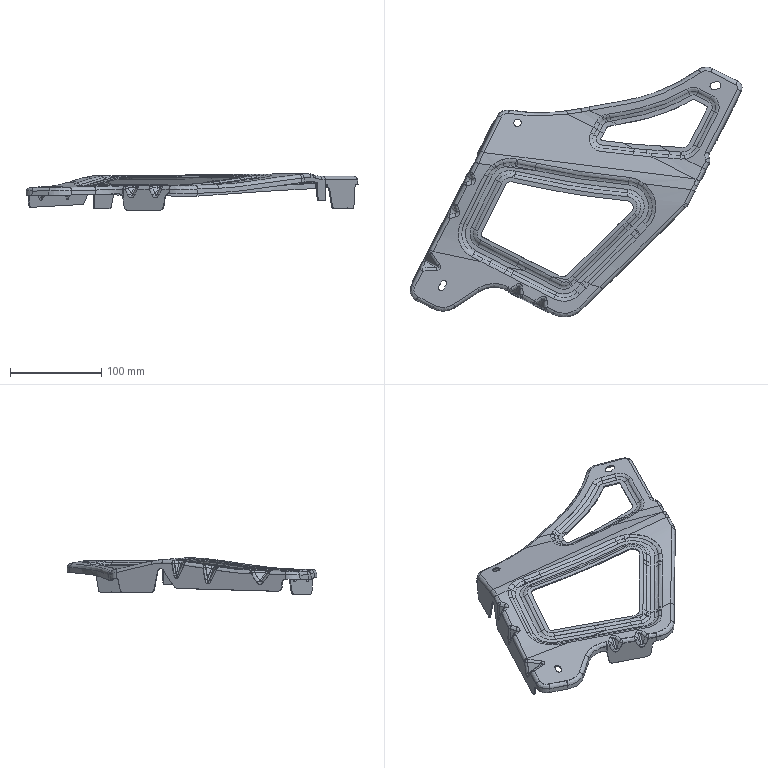Part | STEP file | 9805823280.1BPIECE_SOLIDE_FINALE_id38_x_t | 1 solid | 628 faces | box 364.658 x 274.569 x 40.313 mm | volume 68890 mm3 | spline 454 | cylinder 84 | plane 43 | other 27 | sphere 20 | commonest cylinder face diameters 5.5 x29 8 x23 3 x6 8.2 x4 4 x2 6 x2